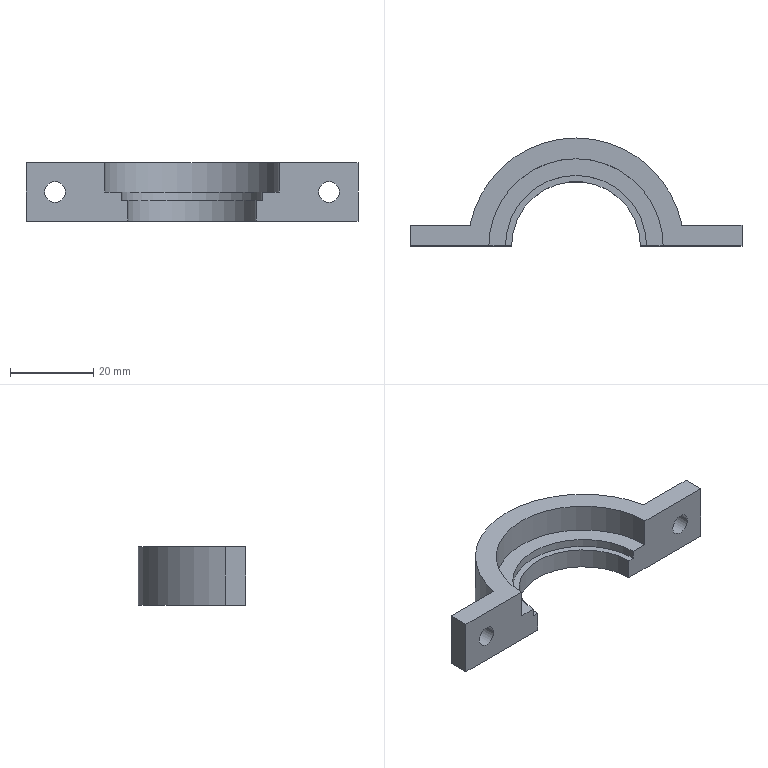Part | SolidWorks | features BaseBody 1 | 1 solid | 18 faces | box 80 x 26 x 14 mm | volume 9008 mm3 | plane 10 | cylinder 8 | commonest cylinder face diameters 5 x4 31 x1 34 x1 42 x1 52 x1
STEP:
#1=CARTESIAN_POINT('',(-30.5,0.,7.));
#2=VERTEX_POINT('',#1);
#3=CARTESIAN_POINT('',(-35.5,0.,7.));
#4=VERTEX_POINT('',#3);
#5=CARTESIAN_POINT('',(-33.,0.,7.));
#6=DIRECTION('',(0.,1.,0.));
#7=DIRECTION('',(-1.,0.,0.));
#8=AXIS2_PLACEMENT_3D('',#5,#6,#7);
#9=CIRCLE('',#8,2.5);
#10=EDGE_CURVE('',#2,#4,#9,.T.);
#11=ORIENTED_EDGE('',*,*,#10,.F.);
#12=CARTESIAN_POINT('',(-30.5,5.,7.));
#13=VERTEX_POINT('',#12);
#14=CARTESIAN_POINT('',(-30.5,5.,7.));
#15=DIRECTION('',(0.,1.,0.));
#16=VECTOR('',#15,1000.);
#17=LINE('',#14,#16);
#18=EDGE_CURVE('',#2,#13,#17,.T.);
#19=ORIENTED_EDGE('',*,*,#18,.T.);
#20=CARTESIAN_POINT('',(-35.5,5.,7.));
#21=VERTEX_POINT('',#20);
#22=CARTESIAN_POINT('',(-33.,5.,7.));
#23=DIRECTION('',(0.,-1.,0.));
#24=DIRECTION('',(-1.,0.,0.));
#25=AXIS2_PLACEMENT_3D('',#22,#23,#24);
#26=CIRCLE('',#25,2.5);
#27=EDGE_CURVE('',#21,#13,#26,.T.);
#28=ORIENTED_EDGE('',*,*,#27,.F.);
#29=CARTESIAN_POINT('',(-35.5,5.,7.));
#30=DIRECTION('',(0.,1.,0.));
#31=VECTOR('',#30,1000.);
#32=LINE('',#29,#31);
#33=EDGE_CURVE('',#4,#21,#32,.T.);
#34=ORIENTED_EDGE('',*,*,#33,.F.);
#35=EDGE_LOOP('',(#11,#19,#28,#34));
#36=FACE_OUTER_BOUND('',#35,.T.);
#37=CARTESIAN_POINT('',(-33.,5.,7.));
#38=DIRECTION('',(0.,1.,0.));
#39=DIRECTION('',(-1.,0.,0.));
#40=AXIS2_PLACEMENT_3D('',#37,#38,#39);
#41=CYLINDRICAL_SURFACE('',#40,2.5);
#42=ADVANCED_FACE('',(#36),#41,.F.);
#43=CARTESIAN_POINT('',(35.5,0.,7.));
#44=VERTEX_POINT('',#43);
#45=CARTESIAN_POINT('',(30.5,0.,7.));
#46=VERTEX_POINT('',#45);
#47=CARTESIAN_POINT('',(33.,0.,7.));
#48=DIRECTION('',(0.,1.,0.));
#49=DIRECTION('',(-1.,0.,0.));
#50=AXIS2_PLACEMENT_3D('',#47,#48,#49);
#51=CIRCLE('',#50,2.5);
#52=EDGE_CURVE('',#44,#46,#51,.T.);
#53=ORIENTED_EDGE('',*,*,#52,.F.);
#54=CARTESIAN_POINT('',(35.5,5.,7.));
#55=VERTEX_POINT('',#54);
#56=CARTESIAN_POINT('',(35.5,5.,7.));
#57=DIRECTION('',(0.,1.,0.));
#58=VECTOR('',#57,1000.);
#59=LINE('',#56,#58);
#60=EDGE_CURVE('',#44,#55,#59,.T.);
#61=ORIENTED_EDGE('',*,*,#60,.T.);
#62=CARTESIAN_POINT('',(30.5,5.,7.));
#63=VERTEX_POINT('',#62);
#64=CARTESIAN_POINT('',(33.,5.,7.));
#65=DIRECTION('',(0.,-1.,0.));
#66=DIRECTION('',(-1.,0.,0.));
#67=AXIS2_PLACEMENT_3D('',#64,#65,#66);
#68=CIRCLE('',#67,2.5);
#69=EDGE_CURVE('',#63,#55,#68,.T.);
#70=ORIENTED_EDGE('',*,*,#69,.F.);
#71=CARTESIAN_POINT('',(30.5,5.,7.));
#72=DIRECTION('',(0.,1.,0.));
#73=VECTOR('',#72,1000.);
#74=LINE('',#71,#73);
#75=EDGE_CURVE('',#46,#63,#74,.T.);
#76=ORIENTED_EDGE('',*,*,#75,.F.);
#77=EDGE_LOOP('',(#53,#61,#70,#76));
#78=FACE_OUTER_BOUND('',#77,.T.);
#79=CARTESIAN_POINT('',(33.,5.,7.));
#80=DIRECTION('',(0.,1.,0.));
#81=DIRECTION('',(-1.,0.,0.));
#82=AXIS2_PLACEMENT_3D('',#79,#80,#81);
#83=CYLINDRICAL_SURFACE('',#82,2.5);
#84=ADVANCED_FACE('',(#78),#83,.F.);
#85=CARTESIAN_POINT('',(15.5,0.,5.));
#86=VERTEX_POINT('',#85);
#87=CARTESIAN_POINT('',(15.5,0.,0.));
#88=VERTEX_POINT('',#87);
#89=CARTESIAN_POINT('',(15.5,0.,5.));
#90=DIRECTION('',(0.,0.,-1.));
#91=VECTOR('',#90,1000.);
#92=LINE('',#89,#91);
#93=EDGE_CURVE('',#86,#88,#92,.T.);
#94=ORIENTED_EDGE('',*,*,#93,.F.);
#95=CARTESIAN_POINT('',(-15.5,0.,5.));
#96=VERTEX_POINT('',#95);
#97=CARTESIAN_POINT('',(0.,0.,5.));
#98=DIRECTION('',(0.,0.,-1.));
#99=DIRECTION('',(-1.,0.,0.));
#100=AXIS2_PLACEMENT_3D('',#97,#98,#99);
#101=CIRCLE('',#100,15.5);
#102=EDGE_CURVE('',#96,#86,#101,.T.);
#103=ORIENTED_EDGE('',*,*,#102,.F.);
#104=CARTESIAN_POINT('',(-15.5,0.,0.));
#105=VERTEX_POINT('',#104);
#106=CARTESIAN_POINT('',(-15.5,0.,5.));
#107=DIRECTION('',(0.,0.,1.));
#108=VECTOR('',#107,1000.);
#109=LINE('',#106,#108);
#110=EDGE_CURVE('',#105,#96,#109,.T.);
#111=ORIENTED_EDGE('',*,*,#110,.F.);
#112=CARTESIAN_POINT('',(0.,0.,0.));
#113=DIRECTION('',(0.,0.,1.));
#114=DIRECTION('',(-1.,0.,0.));
#115=AXIS2_PLACEMENT_3D('',#112,#113,#114);
#116=CIRCLE('',#115,15.5);
#117=EDGE_CURVE('',#88,#105,#116,.T.);
#118=ORIENTED_EDGE('',*,*,#117,.F.);
#119=EDGE_LOOP('',(#94,#103,#111,#118));
#120=FACE_OUTER_BOUND('',#119,.T.);
#121=CARTESIAN_POINT('',(0.,0.,5.));
#122=DIRECTION('',(0.,0.,1.));
#123=DIRECTION('',(-1.,0.,0.));
#124=AXIS2_PLACEMENT_3D('',#121,#122,#123);
#125=CYLINDRICAL_SURFACE('',#124,15.5);
#126=ADVANCED_FACE('',(#120),#125,.F.);
#127=ORIENTED_EDGE('',*,*,#117,.T.);
#128=CARTESIAN_POINT('',(-40.,0.,0.));
#129=VERTEX_POINT('',#128);
#130=CARTESIAN_POINT('',(-40.,0.,0.));
#131=DIRECTION('',(1.,0.,0.));
#132=VECTOR('',#131,1000.);
#133=LINE('',#130,#132);
#134=EDGE_CURVE('',#129,#105,#133,.T.);
#135=ORIENTED_EDGE('',*,*,#134,.F.);
#136=CARTESIAN_POINT('',(-40.,5.,0.));
#137=VERTEX_POINT('',#136);
#138=CARTESIAN_POINT('',(-40.,5.,0.));
#139=DIRECTION('',(0.,-1.,0.));
#140=VECTOR('',#139,1000.);
#141=LINE('',#138,#140);
#142=EDGE_CURVE('',#137,#129,#141,.T.);
#143=ORIENTED_EDGE('',*,*,#142,.F.);
#144=CARTESIAN_POINT('',(-25.515,5.,0.));
#145=VERTEX_POINT('',#144);
#146=CARTESIAN_POINT('',(40.,5.,0.));
#147=DIRECTION('',(-1.,0.,0.));
#148=VECTOR('',#147,1000.);
#149=LINE('',#146,#148);
#150=EDGE_CURVE('',#145,#137,#149,.T.);
#151=ORIENTED_EDGE('',*,*,#150,.F.);
#152=CARTESIAN_POINT('',(25.515,5.,0.));
#153=VERTEX_POINT('',#152);
#154=CARTESIAN_POINT('',(0.,0.,0.));
#155=DIRECTION('',(0.,0.,1.));
#156=DIRECTION('',(1.,0.,0.));
#157=AXIS2_PLACEMENT_3D('',#154,#155,#156);
#158=CIRCLE('',#157,26.);
#159=EDGE_CURVE('',#153,#145,#158,.T.);
#160=ORIENTED_EDGE('',*,*,#159,.F.);
#161=CARTESIAN_POINT('',(40.,5.,0.));
#162=VERTEX_POINT('',#161);
#163=CARTESIAN_POINT('',(40.,5.,0.));
#164=DIRECTION('',(-1.,0.,0.));
#165=VECTOR('',#164,1000.);
#166=LINE('',#163,#165);
#167=EDGE_CURVE('',#162,#153,#166,.T.);
#168=ORIENTED_EDGE('',*,*,#167,.F.);
#169=CARTESIAN_POINT('',(40.,0.,0.));
#170=VERTEX_POINT('',#169);
#171=CARTESIAN_POINT('',(40.,0.,0.));
#172=DIRECTION('',(0.,1.,0.));
#173=VECTOR('',#172,1000.);
#174=LINE('',#171,#173);
#175=EDGE_CURVE('',#170,#162,#174,.T.);
#176=ORIENTED_EDGE('',*,*,#175,.F.);
#177=CARTESIAN_POINT('',(-40.,0.,0.));
#178=DIRECTION('',(1.,0.,0.));
#179=VECTOR('',#178,1000.);
#180=LINE('',#177,#179);
#181=EDGE_CURVE('',#88,#170,#180,.T.);
#182=ORIENTED_EDGE('',*,*,#181,.F.);
#183=EDGE_LOOP('',(#127,#135,#143,#151,#160,#168,#176,#182));
#184=FACE_OUTER_BOUND('',#183,.T.);
#185=CARTESIAN_POINT('',(0.,2.5,0.));
#186=DIRECTION('',(0.,0.,1.));
#187=DIRECTION('',(1.,0.,0.));
#188=AXIS2_PLACEMENT_3D('',#185,#186,#187);
#189=PLANE('',#188);
#190=ADVANCED_FACE('',(#184),#189,.F.);
#191=CARTESIAN_POINT('',(-33.,0.,7.));
#192=DIRECTION('',(0.,1.,0.));
#193=DIRECTION('',(-1.,0.,0.));
#194=AXIS2_PLACEMENT_3D('',#191,#192,#193);
#195=CIRCLE('',#194,2.5);
#196=EDGE_CURVE('',#4,#2,#195,.T.);
#197=ORIENTED_EDGE('',*,*,#196,.T.);
#198=ORIENTED_EDGE('',*,*,#10,.T.);
#199=EDGE_LOOP('',(#197,#198));
#200=FACE_BOUND('',#199,.T.);
#201=ORIENTED_EDGE('',*,*,#110,.T.);
#202=CARTESIAN_POINT('',(-17.,0.,5.));
#203=VERTEX_POINT('',#202);
#204=CARTESIAN_POINT('',(-20.,0.,5.));
#205=DIRECTION('',(-1.,0.,0.));
#206=VECTOR('',#205,1000.);
#207=LINE('',#204,#206);
#208=EDGE_CURVE('',#96,#203,#207,.T.);
#209=ORIENTED_EDGE('',*,*,#208,.T.);
#210=CARTESIAN_POINT('',(-17.,0.,7.));
#211=VERTEX_POINT('',#210);
#212=CARTESIAN_POINT('',(-17.,0.,7.));
#213=DIRECTION('',(0.,0.,1.));
#214=VECTOR('',#213,1000.);
#215=LINE('',#212,#214);
#216=EDGE_CURVE('',#203,#211,#215,.T.);
#217=ORIENTED_EDGE('',*,*,#216,.T.);
#218=CARTESIAN_POINT('',(-21.,0.,7.));
#219=VERTEX_POINT('',#218);
#220=CARTESIAN_POINT('',(-20.,0.,7.));
#221=DIRECTION('',(-1.,0.,0.));
#222=VECTOR('',#221,1000.);
#223=LINE('',#220,#222);
#224=EDGE_CURVE('',#211,#219,#223,.T.);
#225=ORIENTED_EDGE('',*,*,#224,.T.);
#226=CARTESIAN_POINT('',(-21.,0.,14.));
#227=VERTEX_POINT('',#226);
#228=CARTESIAN_POINT('',(-21.,0.,14.));
#229=DIRECTION('',(0.,0.,1.));
#230=VECTOR('',#229,1000.);
#231=LINE('',#228,#230);
#232=EDGE_CURVE('',#219,#227,#231,.T.);
#233=ORIENTED_EDGE('',*,*,#232,.T.);
#234=CARTESIAN_POINT('',(-40.,0.,14.));
#235=VERTEX_POINT('',#234);
#236=CARTESIAN_POINT('',(-40.,0.,14.));
#237=DIRECTION('',(1.,0.,0.));
#238=VECTOR('',#237,1000.);
#239=LINE('',#236,#238);
#240=EDGE_CURVE('',#235,#227,#239,.T.);
#241=ORIENTED_EDGE('',*,*,#240,.F.);
#242=CARTESIAN_POINT('',(-40.,0.,0.));
#243=DIRECTION('',(0.,0.,1.));
#244=VECTOR('',#243,1000.);
#245=LINE('',#242,#244);
#246=EDGE_CURVE('',#129,#235,#245,.T.);
#247=ORIENTED_EDGE('',*,*,#246,.F.);
#248=ORIENTED_EDGE('',*,*,#134,.T.);
#249=EDGE_LOOP('',(#201,#209,#217,#225,#233,#241,#247,#248));
#250=FACE_OUTER_BOUND('',#249,.T.);
#251=CARTESIAN_POINT('',(-40.,0.,0.));
#252=DIRECTION('',(0.,-1.,0.));
#253=DIRECTION('',(0.,0.,-1.));
#254=AXIS2_PLACEMENT_3D('',#251,#252,#253);
#255=PLANE('',#254);
#256=ADVANCED_FACE('',(#200,#250),#255,.T.);
#257=ORIENTED_EDGE('',*,*,#102,.T.);
#258=CARTESIAN_POINT('',(17.,0.,5.));
#259=VERTEX_POINT('',#258);
#260=CARTESIAN_POINT('',(-20.,0.,5.));
#261=DIRECTION('',(-1.,0.,0.));
#262=VECTOR('',#261,1000.);
#263=LINE('',#260,#262);
#264=EDGE_CURVE('',#259,#86,#263,.T.);
#265=ORIENTED_EDGE('',*,*,#264,.F.);
#266=CARTESIAN_POINT('',(0.,0.,5.));
#267=DIRECTION('',(0.,0.,-1.));
#268=DIRECTION('',(-1.,0.,0.));
#269=AXIS2_PLACEMENT_3D('',#266,#267,#268);
#270=CIRCLE('',#269,17.);
#271=EDGE_CURVE('',#203,#259,#270,.T.);
#272=ORIENTED_EDGE('',*,*,#271,.F.);
#273=ORIENTED_EDGE('',*,*,#208,.F.);
#274=EDGE_LOOP('',(#257,#265,#272,#273));
#275=FACE_OUTER_BOUND('',#274,.T.);
#276=CARTESIAN_POINT('',(0.,0.,5.));
#277=DIRECTION('',(0.,0.,1.));
#278=DIRECTION('',(1.,0.,0.));
#279=AXIS2_PLACEMENT_3D('',#276,#277,#278);
#280=PLANE('',#279);
#281=ADVANCED_FACE('',(#275),#280,.T.);
#282=CARTESIAN_POINT('',(17.,0.,7.));
#283=VERTEX_POINT('',#282);
#284=CARTESIAN_POINT('',(17.,0.,7.));
#285=DIRECTION('',(0.,0.,-1.));
#286=VECTOR('',#285,1000.);
#287=LINE('',#284,#286);
#288=EDGE_CURVE('',#283,#259,#287,.T.);
#289=ORIENTED_EDGE('',*,*,#288,.F.);
#290=CARTESIAN_POINT('',(0.,0.,7.));
#291=DIRECTION('',(0.,0.,-1.));
#292=DIRECTION('',(-1.,0.,0.));
#293=AXIS2_PLACEMENT_3D('',#290,#291,#292);
#294=CIRCLE('',#293,17.);
#295=EDGE_CURVE('',#211,#283,#294,.T.);
#296=ORIENTED_EDGE('',*,*,#295,.F.);
#297=ORIENTED_EDGE('',*,*,#216,.F.);
#298=ORIENTED_EDGE('',*,*,#271,.T.);
#299=EDGE_LOOP('',(#289,#296,#297,#298));
#300=FACE_OUTER_BOUND('',#299,.T.);
#301=CARTESIAN_POINT('',(0.,0.,7.));
#302=DIRECTION('',(0.,0.,1.));
#303=DIRECTION('',(-1.,0.,0.));
#304=AXIS2_PLACEMENT_3D('',#301,#302,#303);
#305=CYLINDRICAL_SURFACE('',#304,17.);
#306=ADVANCED_FACE('',(#300),#305,.F.);
#307=CARTESIAN_POINT('',(33.,0.,7.));
#308=DIRECTION('',(0.,1.,0.));
#309=DIRECTION('',(-1.,0.,0.));
#310=AXIS2_PLACEMENT_3D('',#307,#308,#309);
#311=CIRCLE('',#310,2.5);
#312=EDGE_CURVE('',#46,#44,#311,.T.);
#313=ORIENTED_EDGE('',*,*,#312,.T.);
#314=ORIENTED_EDGE('',*,*,#52,.T.);
#315=EDGE_LOOP('',(#313,#314));
#316=FACE_BOUND('',#315,.T.);
#317=ORIENTED_EDGE('',*,*,#93,.T.);
#318=ORIENTED_EDGE('',*,*,#181,.T.);
#319=CARTESIAN_POINT('',(40.,0.,14.));
#320=VERTEX_POINT('',#319);
#321=CARTESIAN_POINT('',(40.,0.,0.));
#322=DIRECTION('',(0.,0.,1.));
#323=VECTOR('',#322,1000.);
#324=LINE('',#321,#323);
#325=EDGE_CURVE('',#170,#320,#324,.T.);
#326=ORIENTED_EDGE('',*,*,#325,.T.);
#327=CARTESIAN_POINT('',(21.,0.,14.));
#328=VERTEX_POINT('',#327);
#329=CARTESIAN_POINT('',(-40.,0.,14.));
#330=DIRECTION('',(1.,0.,0.));
#331=VECTOR('',#330,1000.);
#332=LINE('',#329,#331);
#333=EDGE_CURVE('',#328,#320,#332,.T.);
#334=ORIENTED_EDGE('',*,*,#333,.F.);
#335=CARTESIAN_POINT('',(21.,0.,7.));
#336=VERTEX_POINT('',#335);
#337=CARTESIAN_POINT('',(21.,0.,14.));
#338=DIRECTION('',(0.,0.,-1.));
#339=VECTOR('',#338,1000.);
#340=LINE('',#337,#339);
#341=EDGE_CURVE('',#328,#336,#340,.T.);
#342=ORIENTED_EDGE('',*,*,#341,.T.);
#343=CARTESIAN_POINT('',(-20.,0.,7.));
#344=DIRECTION('',(-1.,0.,0.));
#345=VECTOR('',#344,1000.);
#346=LINE('',#343,#345);
#347=EDGE_CURVE('',#336,#283,#346,.T.);
#348=ORIENTED_EDGE('',*,*,#347,.T.);
#349=ORIENTED_EDGE('',*,*,#288,.T.);
#350=ORIENTED_EDGE('',*,*,#264,.T.);
#351=EDGE_LOOP('',(#317,#318,#326,#334,#342,#348,#349,#350));
#352=FACE_OUTER_BOUND('',#351,.T.);
#353=CARTESIAN_POINT('',(-40.,0.,0.));
#354=DIRECTION('',(0.,-1.,0.));
#355=DIRECTION('',(0.,0.,-1.));
#356=AXIS2_PLACEMENT_3D('',#353,#354,#355);
#357=PLANE('',#356);
#358=ADVANCED_FACE('',(#316,#352),#357,.T.);
#359=ORIENTED_EDGE('',*,*,#295,.T.);
#360=ORIENTED_EDGE('',*,*,#347,.F.);
#361=CARTESIAN_POINT('',(0.,0.,7.));
#362=DIRECTION('',(0.,0.,-1.));
#363=DIRECTION('',(-1.,0.,0.));
#364=AXIS2_PLACEMENT_3D('',#361,#362,#363);
#365=CIRCLE('',#364,21.);
#366=EDGE_CURVE('',#219,#336,#365,.T.);
#367=ORIENTED_EDGE('',*,*,#366,.F.);
#368=ORIENTED_EDGE('',*,*,#224,.F.);
#369=EDGE_LOOP('',(#359,#360,#367,#368));
#370=FACE_OUTER_BOUND('',#369,.T.);
#371=CARTESIAN_POINT('',(0.,0.,7.));
#372=DIRECTION('',(0.,0.,1.));
#373=DIRECTION('',(1.,0.,0.));
#374=AXIS2_PLACEMENT_3D('',#371,#372,#373);
#375=PLANE('',#374);
#376=ADVANCED_FACE('',(#370),#375,.T.);
#377=ORIENTED_EDGE('',*,*,#341,.F.);
#378=CARTESIAN_POINT('',(0.,0.,14.));
#379=DIRECTION('',(0.,0.,-1.));
#380=DIRECTION('',(-1.,0.,0.));
#381=AXIS2_PLACEMENT_3D('',#378,#379,#380);
#382=CIRCLE('',#381,21.);
#383=EDGE_CURVE('',#227,#328,#382,.T.);
#384=ORIENTED_EDGE('',*,*,#383,.F.);
#385=ORIENTED_EDGE('',*,*,#232,.F.);
#386=ORIENTED_EDGE('',*,*,#366,.T.);
#387=EDGE_LOOP('',(#377,#384,#385,#386));
#388=FACE_OUTER_BOUND('',#387,.T.);
#389=CARTESIAN_POINT('',(0.,0.,14.));
#390=DIRECTION('',(0.,0.,1.));
#391=DIRECTION('',(-1.,0.,0.));
#392=AXIS2_PLACEMENT_3D('',#389,#390,#391);
#393=CYLINDRICAL_SURFACE('',#392,21.);
#394=ADVANCED_FACE('',(#388),#393,.F.);
#395=ORIENTED_EDGE('',*,*,#383,.T.);
#396=ORIENTED_EDGE('',*,*,#333,.T.);
#397=CARTESIAN_POINT('',(40.,5.,14.));
#398=VERTEX_POINT('',#397);
#399=CARTESIAN_POINT('',(40.,0.,14.));
#400=DIRECTION('',(0.,1.,0.));
#401=VECTOR('',#400,1000.);
#402=LINE('',#399,#401);
#403=EDGE_CURVE('',#320,#398,#402,.T.);
#404=ORIENTED_EDGE('',*,*,#403,.T.);
#405=CARTESIAN_POINT('',(25.515,5.,14.));
#406=VERTEX_POINT('',#405);
#407=CARTESIAN_POINT('',(40.,5.,14.));
#408=DIRECTION('',(-1.,0.,0.));
#409=VECTOR('',#408,1000.);
#410=LINE('',#407,#409);
#411=EDGE_CURVE('',#398,#406,#410,.T.);
#412=ORIENTED_EDGE('',*,*,#411,.T.);
#413=CARTESIAN_POINT('',(-25.515,5.,14.));
#414=VERTEX_POINT('',#413);
#415=CARTESIAN_POINT('',(0.,0.,14.));
#416=DIRECTION('',(0.,0.,1.));
#417=DIRECTION('',(1.,0.,0.));
#418=AXIS2_PLACEMENT_3D('',#415,#416,#417);
#419=CIRCLE('',#418,26.);
#420=EDGE_CURVE('',#406,#414,#419,.T.);
#421=ORIENTED_EDGE('',*,*,#420,.T.);
#422=CARTESIAN_POINT('',(-40.,5.,14.));
#423=VERTEX_POINT('',#422);
#424=CARTESIAN_POINT('',(40.,5.,14.));
#425=DIRECTION('',(-1.,0.,0.));
#426=VECTOR('',#425,1000.);
#427=LINE('',#424,#426);
#428=EDGE_CURVE('',#414,#423,#427,.T.);
#429=ORIENTED_EDGE('',*,*,#428,.T.);
#430=CARTESIAN_POINT('',(-40.,5.,14.));
#431=DIRECTION('',(0.,-1.,0.));
#432=VECTOR('',#431,1000.);
#433=LINE('',#430,#432);
#434=EDGE_CURVE('',#423,#235,#433,.T.);
#435=ORIENTED_EDGE('',*,*,#434,.T.);
#436=ORIENTED_EDGE('',*,*,#240,.T.);
#437=EDGE_LOOP('',(#395,#396,#404,#412,#421,#429,#435,#436));
#438=FACE_OUTER_BOUND('',#437,.T.);
#439=CARTESIAN_POINT('',(0.,8.953,14.));
#440=DIRECTION('',(0.,0.,1.));
#441=DIRECTION('',(1.,0.,0.));
#442=AXIS2_PLACEMENT_3D('',#439,#440,#441);
#443=PLANE('',#442);
#444=ADVANCED_FACE('',(#438),#443,.T.);
#445=CARTESIAN_POINT('',(-25.515,5.,0.));
#446=DIRECTION('',(0.,0.,-1.));
#447=VECTOR('',#446,1000.);
#448=LINE('',#445,#447);
#449=EDGE_CURVE('',#414,#145,#448,.T.);
#450=ORIENTED_EDGE('',*,*,#449,.F.);
#451=ORIENTED_EDGE('',*,*,#420,.F.);
#452=CARTESIAN_POINT('',(25.515,5.,0.));
#453=DIRECTION('',(0.,0.,1.));
#454=VECTOR('',#453,1000.);
#455=LINE('',#452,#454);
#456=EDGE_CURVE('',#153,#406,#455,.T.);
#457=ORIENTED_EDGE('',*,*,#456,.F.);
#458=ORIENTED_EDGE('',*,*,#159,.T.);
#459=EDGE_LOOP('',(#450,#451,#457,#458));
#460=FACE_OUTER_BOUND('',#459,.T.);
#461=CARTESIAN_POINT('',(0.,0.,0.));
#462=DIRECTION('',(0.,0.,-1.));
#463=DIRECTION('',(1.,0.,0.));
#464=AXIS2_PLACEMENT_3D('',#461,#462,#463);
#465=CYLINDRICAL_SURFACE('',#464,26.);
#466=ADVANCED_FACE('',(#460),#465,.T.);
#467=ORIENTED_EDGE('',*,*,#69,.T.);
#468=CARTESIAN_POINT('',(33.,5.,7.));
#469=DIRECTION('',(0.,-1.,0.));
#470=DIRECTION('',(-1.,0.,0.));
#471=AXIS2_PLACEMENT_3D('',#468,#469,#470);
#472=CIRCLE('',#471,2.5);
#473=EDGE_CURVE('',#55,#63,#472,.T.);
#474=ORIENTED_EDGE('',*,*,#473,.T.);
#475=EDGE_LOOP('',(#467,#474));
#476=FACE_BOUND('',#475,.T.);
#477=ORIENTED_EDGE('',*,*,#456,.T.);
#478=ORIENTED_EDGE('',*,*,#411,.F.);
#479=CARTESIAN_POINT('',(40.,5.,0.));
#480=DIRECTION('',(0.,0.,1.));
#481=VECTOR('',#480,1000.);
#482=LINE('',#479,#481);
#483=EDGE_CURVE('',#162,#398,#482,.T.);
#484=ORIENTED_EDGE('',*,*,#483,.F.);
#485=ORIENTED_EDGE('',*,*,#167,.T.);
#486=EDGE_LOOP('',(#477,#478,#484,#485));
#487=FACE_OUTER_BOUND('',#486,.T.);
#488=CARTESIAN_POINT('',(40.,5.,0.));
#489=DIRECTION('',(0.,1.,0.));
#490=DIRECTION('',(1.,0.,0.));
#491=AXIS2_PLACEMENT_3D('',#488,#489,#490);
#492=PLANE('',#491);
#493=ADVANCED_FACE('',(#476,#487),#492,.T.);
#494=ORIENTED_EDGE('',*,*,#175,.T.);
#495=ORIENTED_EDGE('',*,*,#483,.T.);
#496=ORIENTED_EDGE('',*,*,#403,.F.);
#497=ORIENTED_EDGE('',*,*,#325,.F.);
#498=EDGE_LOOP('',(#494,#495,#496,#497));
#499=FACE_OUTER_BOUND('',#498,.T.);
#500=CARTESIAN_POINT('',(40.,0.,0.));
#501=DIRECTION('',(1.,0.,0.));
#502=DIRECTION('',(0.,-1.,0.));
#503=AXIS2_PLACEMENT_3D('',#500,#501,#502);
#504=PLANE('',#503);
#505=ADVANCED_FACE('',(#499),#504,.T.);
#506=ORIENTED_EDGE('',*,*,#142,.T.);
#507=ORIENTED_EDGE('',*,*,#246,.T.);
#508=ORIENTED_EDGE('',*,*,#434,.F.);
#509=CARTESIAN_POINT('',(-40.,5.,0.));
#510=DIRECTION('',(0.,0.,1.));
#511=VECTOR('',#510,1000.);
#512=LINE('',#509,#511);
#513=EDGE_CURVE('',#137,#423,#512,.T.);
#514=ORIENTED_EDGE('',*,*,#513,.F.);
#515=EDGE_LOOP('',(#506,#507,#508,#514));
#516=FACE_OUTER_BOUND('',#515,.T.);
#517=CARTESIAN_POINT('',(-40.,5.,0.));
#518=DIRECTION('',(-1.,0.,0.));
#519=DIRECTION('',(0.,0.,1.));
#520=AXIS2_PLACEMENT_3D('',#517,#518,#519);
#521=PLANE('',#520);
#522=ADVANCED_FACE('',(#516),#521,.T.);
#523=ORIENTED_EDGE('',*,*,#27,.T.);
#524=CARTESIAN_POINT('',(-33.,5.,7.));
#525=DIRECTION('',(0.,-1.,0.));
#526=DIRECTION('',(-1.,0.,0.));
#527=AXIS2_PLACEMENT_3D('',#524,#525,#526);
#528=CIRCLE('',#527,2.5);
#529=EDGE_CURVE('',#13,#21,#528,.T.);
#530=ORIENTED_EDGE('',*,*,#529,.T.);
#531=EDGE_LOOP('',(#523,#530));
#532=FACE_BOUND('',#531,.T.);
#533=ORIENTED_EDGE('',*,*,#449,.T.);
#534=ORIENTED_EDGE('',*,*,#150,.T.);
#535=ORIENTED_EDGE('',*,*,#513,.T.);
#536=ORIENTED_EDGE('',*,*,#428,.F.);
#537=EDGE_LOOP('',(#533,#534,#535,#536));
#538=FACE_OUTER_BOUND('',#537,.T.);
#539=CARTESIAN_POINT('',(40.,5.,0.));
#540=DIRECTION('',(0.,1.,0.));
#541=DIRECTION('',(1.,0.,0.));
#542=AXIS2_PLACEMENT_3D('',#539,#540,#541);
#543=PLANE('',#542);
#544=ADVANCED_FACE('',(#532,#538),#543,.T.);
#545=ORIENTED_EDGE('',*,*,#60,.F.);
#546=ORIENTED_EDGE('',*,*,#312,.F.);
#547=ORIENTED_EDGE('',*,*,#75,.T.);
#548=ORIENTED_EDGE('',*,*,#473,.F.);
#549=EDGE_LOOP('',(#545,#546,#547,#548));
#550=FACE_OUTER_BOUND('',#549,.T.);
#551=CARTESIAN_POINT('',(33.,5.,7.));
#552=DIRECTION('',(0.,1.,0.));
#553=DIRECTION('',(-1.,0.,0.));
#554=AXIS2_PLACEMENT_3D('',#551,#552,#553);
#555=CYLINDRICAL_SURFACE('',#554,2.5);
#556=ADVANCED_FACE('',(#550),#555,.F.);
#557=ORIENTED_EDGE('',*,*,#18,.F.);
#558=ORIENTED_EDGE('',*,*,#196,.F.);
#559=ORIENTED_EDGE('',*,*,#33,.T.);
#560=ORIENTED_EDGE('',*,*,#529,.F.);
#561=EDGE_LOOP('',(#557,#558,#559,#560));
#562=FACE_OUTER_BOUND('',#561,.T.);
#563=CARTESIAN_POINT('',(-33.,5.,7.));
#564=DIRECTION('',(0.,1.,0.));
#565=DIRECTION('',(-1.,0.,0.));
#566=AXIS2_PLACEMENT_3D('',#563,#564,#565);
#567=CYLINDRICAL_SURFACE('',#566,2.5);
#568=ADVANCED_FACE('',(#562),#567,.F.);
#569=CLOSED_SHELL('',(#42,#84,#126,#190,#256,#281,#306,#358,#376,#394,#444,#466,#493,#505,#522,#544,#556,#568));
#570=MANIFOLD_SOLID_BREP('',#569);
#571=CARTESIAN_POINT('',(0.,0.,0.));
#572=DIRECTION('',(0.,0.,1.));
#573=DIRECTION('',(1.,0.,0.));
#574=AXIS2_PLACEMENT_3D('',#571,#572,#573);
#575=(LENGTH_UNIT()NAMED_UNIT(*)SI_UNIT(.MILLI.,.METRE.));
#576=UNCERTAINTY_MEASURE_WITH_UNIT(LENGTH_MEASURE(0.00001),#575,'','');
#577=(NAMED_UNIT(*)PLANE_ANGLE_UNIT()SI_UNIT($,.RADIAN.));
#578=(NAMED_UNIT(*)SI_UNIT($,.STERADIAN.)SOLID_ANGLE_UNIT());
#579=(GEOMETRIC_REPRESENTATION_CONTEXT(3)GLOBAL_UNCERTAINTY_ASSIGNED_CONTEXT((#576))GLOBAL_UNIT_ASSIGNED_CONTEXT((#575,#577,#578))REPRESENTATION_CONTEXT('',''));
#580=ADVANCED_BREP_SHAPE_REPRESENTATION('',(#570,#574),#579);